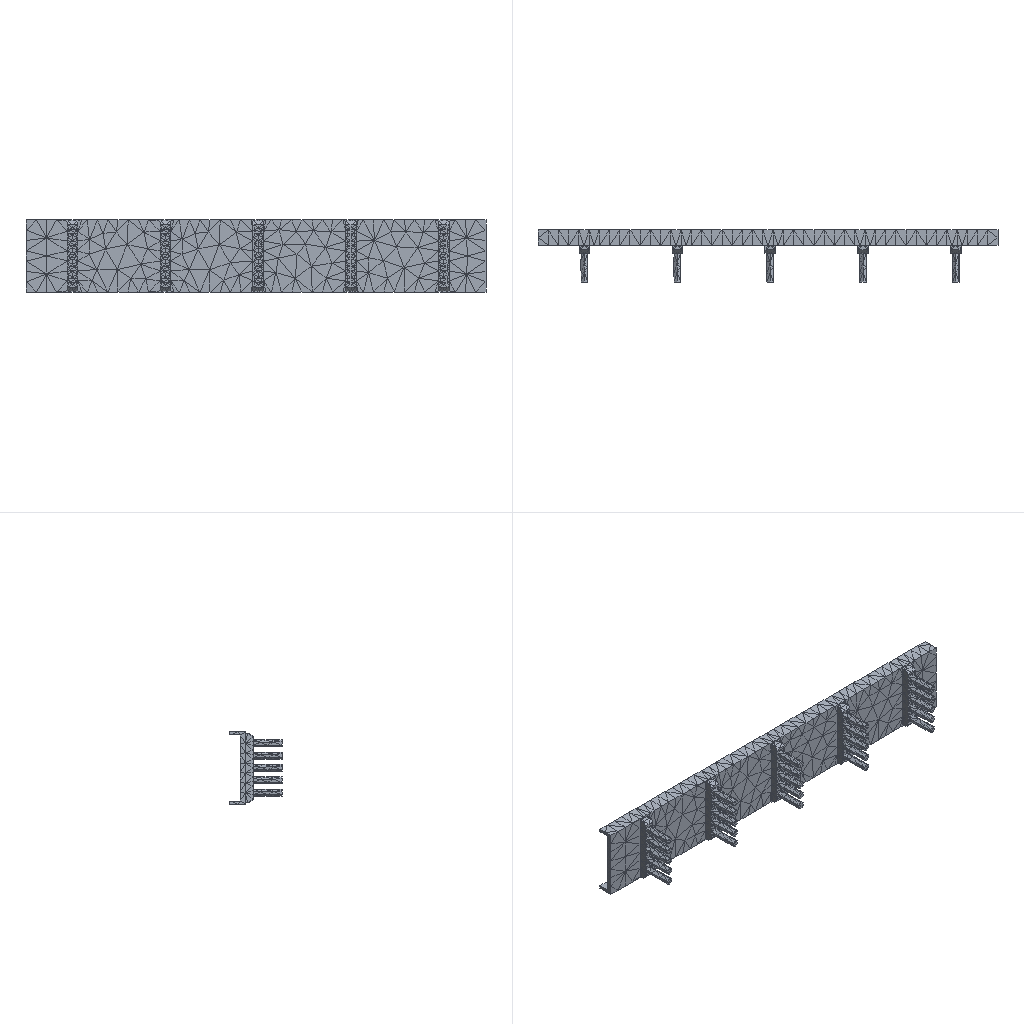Simulation study | ansys workbench
Set-up summary:
category,name,step,type,value,unit,region
solver,ansys_workbench
units,mm-N-s-tonne (MPa),,stated,"/units,MPA"
analysis,LS1,,static
load_step,LS1,LS1,static,nsubst=1; time=1
mesh,nodes,,,7731
mesh,elements,,,3885
element_type,SOLID187,,,3485
element_type,SURF154,,,400
material,C40 Concrete,,E,32500,tonne s^-2 mm^-1
material,C40 Concrete,,nu,0.2
material,C40 Concrete,,density,2.5e-09,tonne mm^-3
material,C40 Concrete,,conductivity,60.5,tonne mm s^-3 C^-1
material,C40 Concrete,,specific_heat,4.34e+08,mm^2 s^-2 C^-1
material,C40 Concrete,,cte,3.25e+10,C^-1
material,C40 Concrete,,permeability,10000
material,C40 Concrete,,resistivity,0.00017,ohm mm
load,Define Force Using Surface Effect Elements,LS1,surface-effect pres face 2,-0.1602,,SURF154 #2
bc,Fixed Supports,model,fixed,[dofs=ALL],,_FIXEDSU
named_set,______,,node,375
named_set,_FIXEDSU,,node,375
Ansys APDL input file, long lists of numbers shortened:
/batch
/config,noeldb,1     ! force off writing results to database
*get,_wallstrt,active,,time,wall
! ANSYS input file written by Workbench version 2022 R1
! File used for geometry attach:
/title,1111111--____ (D5)
! ****** Begin Custom Load Command Snippet ******
/COM, ACT Extensions:
/COM,     LSDYNA, 2021.1
/COM,
! ****** End   Custom Load Command Snippet ******
*DIM,_wb_ProjectScratch_dir,string,248
_wb_ProjectScratch_dir(1) = ''
*DIM,_wb_SolverFiles_dir,string,248
_wb_SolverFiles_dir(1) = ''
*DIM,_wb_userfiles_dir,string,248
_wb_userfiles_dir(1) = ''
/com,--- Data in consistent NMM units. See Solving Units in the help system for more information.
/units,MPA
/nopr
/wb,file,start              !  signify a WB generated input file
/prep7
! Turn off shape checking because checks already performed inside WB mesher.
! See help system for more information.
SHPP,OFF,,NOWARN
/nolist
etcon,set             ! allow ANSYS to choose best KEYOP's for 180x elements, resets any applicable keyopt to MAPDL defaults
/com,*********** Nodes for the whole assembly ***********
nblock,3,,8504
(1i9,3e20.9e3)
        1     1.820893372E+02    -3.555143419E+01     8.500000000E+00
! (7730 more lines like these left out)
-1
/wb,elem,start            !  set before creation of elements
/com,*********** Elements for Body 1 "__3-FreeParts|__(__)1" ***********
et,1,187
eblock,19,solid,,3485
(19i9)
        1        1        1        1        0        0        0        0       10        0        1       14      973     1429       16     1529     6838     1530     1527
! (6969 more lines like these left out)
-1
/wb,elem,end               !  done creating elements
/com,*********** Send User Defined Coordinate System(s) ***********
csys,0
toffst,273.15,  ! Temperature offset from absolute zero
/com,*********** Set Reference Temperature ***********
tref,22.
/wb,mat,start              !  starting to send materials
/com,*********** Send Materials ***********
Temperature = 'TEMP' ! Temperature
MP,DENS,1,2.5e-09,	! tonne mm^-3
MP,ALPX,1,32500000000,	! C^-1
MP,C,1,434000000,	! mm^2 s^-2 C^-1
MP,KXX,1,60.5,	! tonne mm s^-3 C^-1
MP,RSVX,1,0.00017,	! ohm mm
MP,EX,1,32500,	! tonne s^-2 mm^-1
MP,NUXY,1,0.2,
MP,MURX,1,10000,
/wb,mat,end                !  done sending materials
!************************* Model Summary ********************
!__3-FreeParts|__(__)1,	C40混凝土,	matid,	1
!************************* End Model Summary ********************
! get the diagonal of the bounding box. Needed later for other things
*get,_xmin,node,,mnloc,x
*get,_ymin,node,,mnloc,y
*get,_zmin,node,,mnloc,z
*get,_xmax,node,,mxloc,x
*get,_ymax,node,,mxloc,y
*get,_zmax,node,,mxloc,z
_ASMDIAG=(_xmax-_xmin)*(_xmax-_xmin)+(_ymax-_ymin)*(_ymax-_ymin)+(_zmax-_zmin)*(_zmax-_zmin)
_ASMDIAG=SQRT(_ASMDIAG)
/wb,contact,start          !  starting to send contact
/wb,contact,end            !  done creating contacts
/com,*********** Send Named Selection as Node Component ***********
CMBLOCK,______  ,NODE,      375
(8i10)
         1         2         3         4        13        14        15        16
! (46 more lines like these left out)
/golist
/wb,load,start             !  starting to send loads
/com,*********** Fixed Supports ***********
CMBLOCK,_FIXEDSU,NODE,      375
(8i10)
         1         2         3         4        13        14        15        16
! (46 more lines like these left out)
cmsel,s,_FIXEDSU
d,all,all
nsel,all
/com,*********** Define Force Using Surface Effect Elements ***********
local,12,0,0.,0.,0.,0.,0.,0.
csys,0
et,2,154
eblock,10,,,400
(15i9)
     6244        2        2        2       12     1319     1333     1353     1353     7587     7656     1353     7589
! (399 more lines like these left out)
-1
esel,s,type,,2
keyop,2,2,1                ! Apply load in local coordinate system
keyop,2,7,1                ! Use original area so load is constant in large deformation
esel,all
/gst,on,on
fini
*get,_numnode,node,0,count
*get,_numelem,elem,0,count
*get, _MAXELEMNUM, elem, 0, NUM, MAX
*get, _MAXNODENUM, node, 0, NUM, MAX
*get, _MAXELEMTYPE, etyp, 0, NUM, MAX
*get, _MAXREALCONST, real, 0, NUM, MAX
/go
/wb,load,end               !  done creating loads
/com,--- Number of total nodes = %_numnode%
/com,--- Number of contact elements = 400
/com,--- Number of spring elements = 0
/com,--- Number of bearing elements = 0
/com,--- Number of solid elements = 3485
/com,--- Number of condensed parts = 0
/com,--- Number of total elements = %_numelem%
*get,_wallbsol,active,,time,wall
/com,****************************************************************************
/com,*************************    SOLUTION       ********************************
/com,****************************************************************************
/solu
antype,0                   ! static analysis
_thickRatio=  0     ! Ratio of thick parts in the model
eqsl,sparse,,,,,1
cntr,print,1               ! print out contact info and also make no initial contact an error
dmpoption,emat,no             ! Don't combine emat file for DANSYS
dmpoption,esav,no             ! Don't combine esav file for DANSYS
nldiag,cont,iter           ! print out contact info each equilibrium iteration
rescontrol,,none                 ! Do not keep any restart files
/com,****************************************************
/com,******************* SOLVE FOR LS 1 OF 1 ****************
esel,s,type,,2
nsle
sfe,all,1,pres,1,0.
sfe,all,2,pres,1,-0.1602
sfe,all,3,pres,1,0.
nsel,all
esel,all
/nopr
/gopr
nsub,1,1,1
time,1.
outres,erase
outres,all,none
outres,nsol,all,
outres,rsol,all
outres,eangl,all
outres,etmp,all
outres,veng,all
outres,strs,all,
outres,epel,all,
outres,eppl,all,
outres,cont,all,
! *********** WB SOLVE COMMAND ***********
! check interactive state
*get,ANSINTER_,active,,int
*if,ANSINTER_,ne,0,then
/eof
*endif
solve
/com *************** Write FE CONNECTORS *********
CEWRITE,file,ce,,INTE
/com,****************************************************
/com,*************** FINISHED SOLVE FOR LS 1 *************
*get,_wallasol,active,,time,wall
/nopr
*get,_numnode,node,0,count
*get,_numelem,elem,0,count
*get, _MAXELEMNUM, elem, 0, NUM, MAX
*get, _MAXNODENUM, node, 0, NUM, MAX,,,INTERNAL
*get, _MAXELEMTYPE, etyp, 0, NUM, MAX
*get, _MAXREALCONST, real, 0, NUM, MAX
/gopr
/post1
xmlo,ENCODING,ISO-8859-1
xmlo,parm
/xml,parm,xml
fini
/gopr
*get,_walldone,active,,time,wall
_preptime=(_wallbsol-_wallstrt)*3600
_solvtime=(_wallasol-_wallbsol)*3600
_posttime=(_walldone-_wallasol)*3600
_totaltim=(_walldone-_wallstrt)*3600
*get,_dlbratio,active,0,solu,dlbr
*get,_combtime,active,0,solu,comb
*get,_ssmode,active,0,solu,ssmm
*get,_ndofs,active,0,solu,ndof
*get,_sol_end_time,active,0,set,time
*if,_sol_end_time,eq,1.,then
/fclean				!clean distributed files
*endif
/com,--- Total number of nodes = %_numnode%
/com,--- Total number of elements = %_numelem%
/com,--- Element load balance ratio = %_dlbratio%
/com,--- Time to combine distributed files = %_combtime%
/com,--- Sparse memory mode = %_ssmode%
/com,--- Number of DOF = %_ndofs%
/wb,file,end               ! done with WB generated input
Results summary:
result,analyses[0].index,,,1
result,analyses[0].system,,,SYS-1
result,analyses[0].deck,,,deck.dat
result,analyses[0].solve_status,,,completed
result,analyses[0].analysis_type,,,static
result,analyses[0].physics,,,mechanical
result,analyses[0].unit_system,,,"NMM: mm, ton, N, s, mV, mA, degC"
result,analyses[0].n_sets,,,1
result,analyses[0].load_steps[0].set,set=1,,1
result,analyses[0].load_steps[0].time_or_freq,set=1,,1
result,analyses[0].load_steps[0].max_displacement_magnitude,set=1,,0.08753
result,analyses[0].load_steps[0].max_von_mises_nodal,set=1,,15.983
result,analyses[0].load_steps[0].reaction_force_sum_xyz[1],set=1,,3.7212e-09
result,analyses[0].load_steps[0].reaction_force_sum_xyz[2],set=1,,5000
result,analyses[0].load_steps[0].reaction_force_sum_xyz[3],set=1,,-3.094e-10